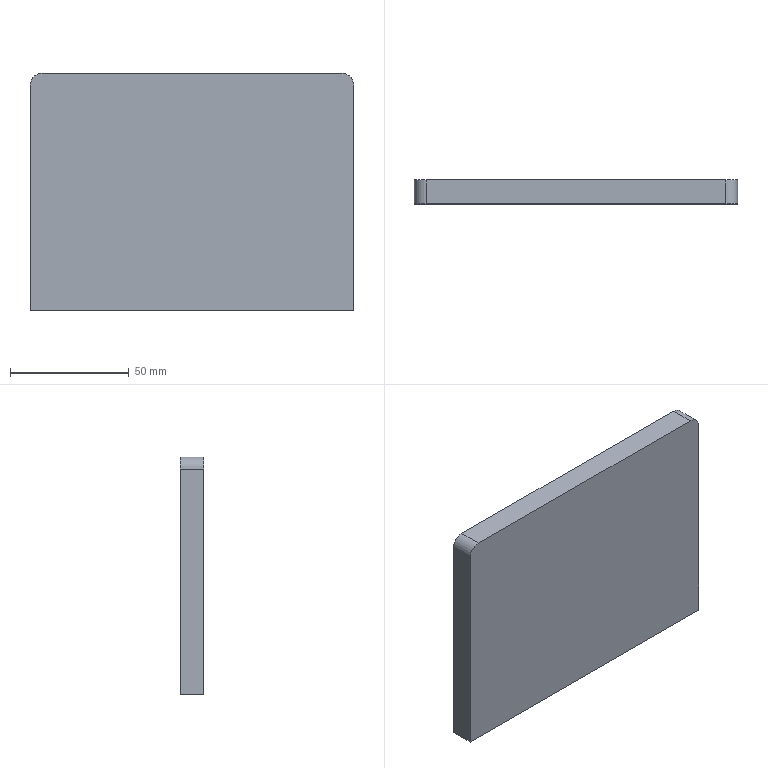Part | STEP file | 1 solid | 8 faces | box 136 x 10 x 100 mm | volume 135893 mm3 | plane 6 | cylinder 2 | commonest cylinder face diameters 10 x2
STEP:
#1=CARTESIAN_POINT('',(0.,0.,0.));
#2=DIRECTION('',(0.,0.,1.));
#3=DIRECTION('',(1.,0.,0.));
#4=AXIS2_PLACEMENT_3D('',#1,#2,#3);
#5=CARTESIAN_POINT('',(-135.863,110.5,353.53));
#6=VERTEX_POINT('',#5);
#7=CARTESIAN_POINT('',(-9.863,110.5,353.53));
#8=VERTEX_POINT('',#7);
#9=CARTESIAN_POINT('',(-72.862,110.5,353.53));
#10=DIRECTION('',(1.,0.,0.));
#11=VECTOR('',#10,1.);
#12=LINE('',#9,#11);
#13=CARTESIAN_POINT('',(-72.862,95.5,353.53));
#14=DIRECTION('',(0.,0.,1.));
#15=DIRECTION('',(1.,0.,0.));
#16=AXIS2_PLACEMENT_3D('',#13,#14,#15);
#17=PLANE('',#16);
#18=CARTESIAN_POINT('',(0.,15.));
#19=DIRECTION('',(1.,0.));
#20=VECTOR('',#19,1.);
#21=LINE('',#18,#20);
#22=(GEOMETRIC_REPRESENTATION_CONTEXT(2)PARAMETRIC_REPRESENTATION_CONTEXT()REPRESENTATION_CONTEXT('',''));
#23=DEFINITIONAL_REPRESENTATION('',(#21),#22);
#24=PCURVE('',#17,#23);
#25=CARTESIAN_POINT('',(-72.862,110.5,253.53));
#26=DIRECTION('',(0.,1.,0.));
#27=DIRECTION('',(0.,0.,1.));
#28=AXIS2_PLACEMENT_3D('',#25,#26,#27);
#29=PLANE('',#28);
#30=CARTESIAN_POINT('',(100.,0.));
#31=DIRECTION('',(0.,1.));
#32=VECTOR('',#31,1.);
#33=LINE('',#30,#32);
#34=(GEOMETRIC_REPRESENTATION_CONTEXT(2)PARAMETRIC_REPRESENTATION_CONTEXT()REPRESENTATION_CONTEXT('',''));
#35=DEFINITIONAL_REPRESENTATION('',(#33),#34);
#36=PCURVE('',#29,#35);
#37=SURFACE_CURVE('',#12,(#24,#36),.PCURVE_S1.);
#38=EDGE_CURVE('',#6,#8,#37,.T.);
#39=ORIENTED_EDGE('',*,*,#38,.F.);
#40=CARTESIAN_POINT('',(-135.863,100.5,353.53));
#41=VERTEX_POINT('',#40);
#42=CARTESIAN_POINT('',(-135.863,95.5,353.53));
#43=DIRECTION('',(0.,-1.,0.));
#44=VECTOR('',#43,1.);
#45=LINE('',#42,#44);
#46=CARTESIAN_POINT('',(-63.,0.));
#47=DIRECTION('',(0.,-1.));
#48=VECTOR('',#47,1.);
#49=LINE('',#46,#48);
#50=(GEOMETRIC_REPRESENTATION_CONTEXT(2)PARAMETRIC_REPRESENTATION_CONTEXT()REPRESENTATION_CONTEXT('',''));
#51=DEFINITIONAL_REPRESENTATION('',(#49),#50);
#52=PCURVE('',#17,#51);
#53=CARTESIAN_POINT('',(-135.863,95.5,348.53));
#54=DIRECTION('',(0.,1.,0.));
#55=DIRECTION('',(0.,0.,1.));
#56=AXIS2_PLACEMENT_3D('',#53,#54,#55);
#57=CYLINDRICAL_SURFACE('',#56,5.);
#58=CARTESIAN_POINT('',(6.283,0.));
#59=DIRECTION('',(0.,-1.));
#60=VECTOR('',#59,1.);
#61=LINE('',#58,#60);
#62=(GEOMETRIC_REPRESENTATION_CONTEXT(2)PARAMETRIC_REPRESENTATION_CONTEXT()REPRESENTATION_CONTEXT('',''));
#63=DEFINITIONAL_REPRESENTATION('',(#61),#62);
#64=PCURVE('',#57,#63);
#65=SURFACE_CURVE('',#45,(#52,#64),.PCURVE_S1.);
#66=EDGE_CURVE('',#6,#41,#65,.T.);
#67=ORIENTED_EDGE('',*,*,#66,.T.);
#68=CARTESIAN_POINT('',(-9.863,100.5,353.53));
#69=VERTEX_POINT('',#68);
#70=CARTESIAN_POINT('',(-72.862,100.5,353.53));
#71=DIRECTION('',(-1.,0.,0.));
#72=VECTOR('',#71,1.);
#73=LINE('',#70,#72);
#74=CARTESIAN_POINT('',(0.,5.));
#75=DIRECTION('',(-1.,0.));
#76=VECTOR('',#75,1.);
#77=LINE('',#74,#76);
#78=(GEOMETRIC_REPRESENTATION_CONTEXT(2)PARAMETRIC_REPRESENTATION_CONTEXT()REPRESENTATION_CONTEXT('',''));
#79=DEFINITIONAL_REPRESENTATION('',(#77),#78);
#80=PCURVE('',#17,#79);
#81=CARTESIAN_POINT('',(-72.862,100.5,253.53));
#82=DIRECTION('',(0.,1.,0.));
#83=DIRECTION('',(0.,0.,1.));
#84=AXIS2_PLACEMENT_3D('',#81,#82,#83);
#85=PLANE('',#84);
#86=CARTESIAN_POINT('',(100.,0.));
#87=DIRECTION('',(0.,-1.));
#88=VECTOR('',#87,1.);
#89=LINE('',#86,#88);
#90=(GEOMETRIC_REPRESENTATION_CONTEXT(2)PARAMETRIC_REPRESENTATION_CONTEXT()REPRESENTATION_CONTEXT('',''));
#91=DEFINITIONAL_REPRESENTATION('',(#89),#90);
#92=PCURVE('',#85,#91);
#93=SURFACE_CURVE('',#73,(#80,#92),.PCURVE_S1.);
#94=EDGE_CURVE('',#69,#41,#93,.T.);
#95=ORIENTED_EDGE('',*,*,#94,.F.);
#96=CARTESIAN_POINT('',(-9.863,95.5,353.53));
#97=DIRECTION('',(0.,1.,0.));
#98=VECTOR('',#97,1.);
#99=LINE('',#96,#98);
#100=CARTESIAN_POINT('',(63.,0.));
#101=DIRECTION('',(0.,1.));
#102=VECTOR('',#101,1.);
#103=LINE('',#100,#102);
#104=(GEOMETRIC_REPRESENTATION_CONTEXT(2)PARAMETRIC_REPRESENTATION_CONTEXT()REPRESENTATION_CONTEXT('',''));
#105=DEFINITIONAL_REPRESENTATION('',(#103),#104);
#106=PCURVE('',#17,#105);
#107=CARTESIAN_POINT('',(-9.863,95.5,348.53));
#108=DIRECTION('',(0.,-1.,0.));
#109=DIRECTION('',(0.,0.,-1.));
#110=AXIS2_PLACEMENT_3D('',#107,#108,#109);
#111=CYLINDRICAL_SURFACE('',#110,5.);
#112=CARTESIAN_POINT('',(3.142,0.));
#113=DIRECTION('',(0.,-1.));
#114=VECTOR('',#113,1.);
#115=LINE('',#112,#114);
#116=(GEOMETRIC_REPRESENTATION_CONTEXT(2)PARAMETRIC_REPRESENTATION_CONTEXT()REPRESENTATION_CONTEXT('',''));
#117=DEFINITIONAL_REPRESENTATION('',(#115),#116);
#118=PCURVE('',#111,#117);
#119=SURFACE_CURVE('',#99,(#106,#118),.PCURVE_S1.);
#120=EDGE_CURVE('',#69,#8,#119,.T.);
#121=ORIENTED_EDGE('',*,*,#120,.T.);
#122=EDGE_LOOP('',(#39,#67,#95,#121));
#123=FACE_BOUND('',#122,.T.);
#124=ADVANCED_FACE('',(#123),#17,.T.);
#125=ORIENTED_EDGE('',*,*,#94,.T.);
#126=CARTESIAN_POINT('',(-140.863,100.5,348.53));
#127=VERTEX_POINT('',#126);
#128=CARTESIAN_POINT('',(-135.863,100.5,348.53));
#129=DIRECTION('',(0.,-1.,0.));
#130=DIRECTION('',(0.,0.,1.));
#131=AXIS2_PLACEMENT_3D('',#128,#129,#130);
#132=CIRCLE('',#131,5.);
#133=CARTESIAN_POINT('',(100.,-63.));
#134=CARTESIAN_POINT('',(100.,-71.66));
#135=CARTESIAN_POINT('',(92.5,-67.33));
#136=CARTESIAN_POINT('',(85.,-63.));
#137=CARTESIAN_POINT('',(92.5,-58.67));
#138=CARTESIAN_POINT('',(100.,-54.34));
#139=CARTESIAN_POINT('',(100.,-63.));
#140=(BOUNDED_CURVE()B_SPLINE_CURVE(2,(#133,#134,#135,#136,#137,#138,#139),.UNSPECIFIED.,.T.,.F.)B_SPLINE_CURVE_WITH_KNOTS((1,2,2,2,2,1),(-2.094,0.,2.094,4.189,6.283,8.378),.UNSPECIFIED.)CURVE()GEOMETRIC_REPRESENTATION_ITEM()RATIONAL_B_SPLINE_CURVE((1.,0.5,1.,0.5,1.,0.5,1.))REPRESENTATION_ITEM(''));
#141=(GEOMETRIC_REPRESENTATION_CONTEXT(2)PARAMETRIC_REPRESENTATION_CONTEXT()REPRESENTATION_CONTEXT('',''));
#142=DEFINITIONAL_REPRESENTATION('',(#140),#141);
#143=PCURVE('',#85,#142);
#144=CARTESIAN_POINT('',(6.283,5.));
#145=DIRECTION('',(-1.,0.));
#146=VECTOR('',#145,1.);
#147=LINE('',#144,#146);
#148=(GEOMETRIC_REPRESENTATION_CONTEXT(2)PARAMETRIC_REPRESENTATION_CONTEXT()REPRESENTATION_CONTEXT('',''));
#149=DEFINITIONAL_REPRESENTATION('',(#147),#148);
#150=PCURVE('',#57,#149);
#151=SURFACE_CURVE('',#132,(#143,#150),.PCURVE_S1.);
#152=EDGE_CURVE('',#41,#127,#151,.T.);
#153=ORIENTED_EDGE('',*,*,#152,.T.);
#154=CARTESIAN_POINT('',(-140.863,100.5,253.53));
#155=VERTEX_POINT('',#154);
#156=CARTESIAN_POINT('',(-140.863,100.5,253.53));
#157=DIRECTION('',(0.,0.,1.));
#158=VECTOR('',#157,1.);
#159=LINE('',#156,#158);
#160=CARTESIAN_POINT('',(0.,-68.));
#161=DIRECTION('',(1.,0.));
#162=VECTOR('',#161,1.);
#163=LINE('',#160,#162);
#164=(GEOMETRIC_REPRESENTATION_CONTEXT(2)PARAMETRIC_REPRESENTATION_CONTEXT()REPRESENTATION_CONTEXT('',''));
#165=DEFINITIONAL_REPRESENTATION('',(#163),#164);
#166=PCURVE('',#85,#165);
#167=CARTESIAN_POINT('',(-140.863,95.5,253.53));
#168=DIRECTION('',(-1.,0.,0.));
#169=DIRECTION('',(0.,0.,1.));
#170=AXIS2_PLACEMENT_3D('',#167,#168,#169);
#171=PLANE('',#170);
#172=CARTESIAN_POINT('',(0.,5.));
#173=DIRECTION('',(1.,0.));
#174=VECTOR('',#173,1.);
#175=LINE('',#172,#174);
#176=(GEOMETRIC_REPRESENTATION_CONTEXT(2)PARAMETRIC_REPRESENTATION_CONTEXT()REPRESENTATION_CONTEXT('',''));
#177=DEFINITIONAL_REPRESENTATION('',(#175),#176);
#178=PCURVE('',#171,#177);
#179=SURFACE_CURVE('',#159,(#166,#178),.PCURVE_S1.);
#180=EDGE_CURVE('',#155,#127,#179,.T.);
#181=ORIENTED_EDGE('',*,*,#180,.F.);
#182=CARTESIAN_POINT('',(-4.862,100.5,253.53));
#183=VERTEX_POINT('',#182);
#184=CARTESIAN_POINT('',(-72.862,100.5,253.53));
#185=DIRECTION('',(1.,0.,0.));
#186=VECTOR('',#185,1.);
#187=LINE('',#184,#186);
#188=CARTESIAN_POINT('',(0.,0.));
#189=DIRECTION('',(0.,1.));
#190=VECTOR('',#189,1.);
#191=LINE('',#188,#190);
#192=(GEOMETRIC_REPRESENTATION_CONTEXT(2)PARAMETRIC_REPRESENTATION_CONTEXT()REPRESENTATION_CONTEXT('',''));
#193=DEFINITIONAL_REPRESENTATION('',(#191),#192);
#194=PCURVE('',#85,#193);
#195=CARTESIAN_POINT('',(-72.862,95.5,253.53));
#196=DIRECTION('',(0.,0.,-1.));
#197=DIRECTION('',(-1.,0.,0.));
#198=AXIS2_PLACEMENT_3D('',#195,#196,#197);
#199=PLANE('',#198);
#200=CARTESIAN_POINT('',(0.,5.));
#201=DIRECTION('',(-1.,0.));
#202=VECTOR('',#201,1.);
#203=LINE('',#200,#202);
#204=(GEOMETRIC_REPRESENTATION_CONTEXT(2)PARAMETRIC_REPRESENTATION_CONTEXT()REPRESENTATION_CONTEXT('',''));
#205=DEFINITIONAL_REPRESENTATION('',(#203),#204);
#206=PCURVE('',#199,#205);
#207=SURFACE_CURVE('',#187,(#194,#206),.PCURVE_S1.);
#208=EDGE_CURVE('',#155,#183,#207,.T.);
#209=ORIENTED_EDGE('',*,*,#208,.T.);
#210=CARTESIAN_POINT('',(-4.862,100.5,348.53));
#211=VERTEX_POINT('',#210);
#212=CARTESIAN_POINT('',(-4.862,100.5,253.53));
#213=DIRECTION('',(0.,0.,1.));
#214=VECTOR('',#213,1.);
#215=LINE('',#212,#214);
#216=CARTESIAN_POINT('',(0.,68.));
#217=DIRECTION('',(1.,0.));
#218=VECTOR('',#217,1.);
#219=LINE('',#216,#218);
#220=(GEOMETRIC_REPRESENTATION_CONTEXT(2)PARAMETRIC_REPRESENTATION_CONTEXT()REPRESENTATION_CONTEXT('',''));
#221=DEFINITIONAL_REPRESENTATION('',(#219),#220);
#222=PCURVE('',#85,#221);
#223=CARTESIAN_POINT('',(-4.862,95.5,253.53));
#224=DIRECTION('',(1.,0.,0.));
#225=DIRECTION('',(0.,0.,-1.));
#226=AXIS2_PLACEMENT_3D('',#223,#224,#225);
#227=PLANE('',#226);
#228=CARTESIAN_POINT('',(0.,5.));
#229=DIRECTION('',(-1.,0.));
#230=VECTOR('',#229,1.);
#231=LINE('',#228,#230);
#232=(GEOMETRIC_REPRESENTATION_CONTEXT(2)PARAMETRIC_REPRESENTATION_CONTEXT()REPRESENTATION_CONTEXT('',''));
#233=DEFINITIONAL_REPRESENTATION('',(#231),#232);
#234=PCURVE('',#227,#233);
#235=SURFACE_CURVE('',#215,(#222,#234),.PCURVE_S1.);
#236=EDGE_CURVE('',#183,#211,#235,.T.);
#237=ORIENTED_EDGE('',*,*,#236,.T.);
#238=CARTESIAN_POINT('',(-9.863,100.5,348.53));
#239=DIRECTION('',(0.,-1.,0.));
#240=DIRECTION('',(0.,0.,1.));
#241=AXIS2_PLACEMENT_3D('',#238,#239,#240);
#242=CIRCLE('',#241,5.);
#243=CARTESIAN_POINT('',(100.,63.));
#244=CARTESIAN_POINT('',(100.,54.34));
#245=CARTESIAN_POINT('',(92.5,58.67));
#246=CARTESIAN_POINT('',(85.,63.));
#247=CARTESIAN_POINT('',(92.5,67.33));
#248=CARTESIAN_POINT('',(100.,71.66));
#249=CARTESIAN_POINT('',(100.,63.));
#250=(BOUNDED_CURVE()B_SPLINE_CURVE(2,(#243,#244,#245,#246,#247,#248,#249),.UNSPECIFIED.,.T.,.F.)B_SPLINE_CURVE_WITH_KNOTS((1,2,2,2,2,1),(-2.094,0.,2.094,4.189,6.283,8.378),.UNSPECIFIED.)CURVE()GEOMETRIC_REPRESENTATION_ITEM()RATIONAL_B_SPLINE_CURVE((1.,0.5,1.,0.5,1.,0.5,1.))REPRESENTATION_ITEM(''));
#251=(GEOMETRIC_REPRESENTATION_CONTEXT(2)PARAMETRIC_REPRESENTATION_CONTEXT()REPRESENTATION_CONTEXT('',''));
#252=DEFINITIONAL_REPRESENTATION('',(#250),#251);
#253=PCURVE('',#85,#252);
#254=CARTESIAN_POINT('',(-3.142,-5.));
#255=DIRECTION('',(1.,0.));
#256=VECTOR('',#255,1.);
#257=LINE('',#254,#256);
#258=(GEOMETRIC_REPRESENTATION_CONTEXT(2)PARAMETRIC_REPRESENTATION_CONTEXT()REPRESENTATION_CONTEXT('',''));
#259=DEFINITIONAL_REPRESENTATION('',(#257),#258);
#260=PCURVE('',#111,#259);
#261=SURFACE_CURVE('',#242,(#253,#260),.PCURVE_S1.);
#262=EDGE_CURVE('',#211,#69,#261,.T.);
#263=ORIENTED_EDGE('',*,*,#262,.T.);
#264=EDGE_LOOP('',(#125,#153,#181,#209,#237,#263));
#265=FACE_BOUND('',#264,.T.);
#266=ADVANCED_FACE('',(#265),#85,.F.);
#267=ORIENTED_EDGE('',*,*,#180,.T.);
#268=CARTESIAN_POINT('',(-140.863,110.5,348.53));
#269=VERTEX_POINT('',#268);
#270=CARTESIAN_POINT('',(-140.863,95.5,348.53));
#271=DIRECTION('',(0.,1.,0.));
#272=VECTOR('',#271,1.);
#273=LINE('',#270,#272);
#274=CARTESIAN_POINT('',(95.,0.));
#275=DIRECTION('',(0.,1.));
#276=VECTOR('',#275,1.);
#277=LINE('',#274,#276);
#278=(GEOMETRIC_REPRESENTATION_CONTEXT(2)PARAMETRIC_REPRESENTATION_CONTEXT()REPRESENTATION_CONTEXT('',''));
#279=DEFINITIONAL_REPRESENTATION('',(#277),#278);
#280=PCURVE('',#171,#279);
#281=CARTESIAN_POINT('',(4.712,0.));
#282=DIRECTION('',(0.,1.));
#283=VECTOR('',#282,1.);
#284=LINE('',#281,#283);
#285=(GEOMETRIC_REPRESENTATION_CONTEXT(2)PARAMETRIC_REPRESENTATION_CONTEXT()REPRESENTATION_CONTEXT('',''));
#286=DEFINITIONAL_REPRESENTATION('',(#284),#285);
#287=PCURVE('',#57,#286);
#288=SURFACE_CURVE('',#273,(#280,#287),.PCURVE_S1.);
#289=EDGE_CURVE('',#127,#269,#288,.T.);
#290=ORIENTED_EDGE('',*,*,#289,.T.);
#291=CARTESIAN_POINT('',(-140.863,110.5,253.53));
#292=VERTEX_POINT('',#291);
#293=CARTESIAN_POINT('',(-140.863,110.5,253.53));
#294=DIRECTION('',(0.,0.,1.));
#295=VECTOR('',#294,1.);
#296=LINE('',#293,#295);
#297=CARTESIAN_POINT('',(0.,15.));
#298=DIRECTION('',(1.,0.));
#299=VECTOR('',#298,1.);
#300=LINE('',#297,#299);
#301=(GEOMETRIC_REPRESENTATION_CONTEXT(2)PARAMETRIC_REPRESENTATION_CONTEXT()REPRESENTATION_CONTEXT('',''));
#302=DEFINITIONAL_REPRESENTATION('',(#300),#301);
#303=PCURVE('',#171,#302);
#304=CARTESIAN_POINT('',(0.,-68.));
#305=DIRECTION('',(1.,0.));
#306=VECTOR('',#305,1.);
#307=LINE('',#304,#306);
#308=(GEOMETRIC_REPRESENTATION_CONTEXT(2)PARAMETRIC_REPRESENTATION_CONTEXT()REPRESENTATION_CONTEXT('',''));
#309=DEFINITIONAL_REPRESENTATION('',(#307),#308);
#310=PCURVE('',#29,#309);
#311=SURFACE_CURVE('',#296,(#303,#310),.PCURVE_S1.);
#312=EDGE_CURVE('',#292,#269,#311,.T.);
#313=ORIENTED_EDGE('',*,*,#312,.F.);
#314=CARTESIAN_POINT('',(-140.863,95.5,253.53));
#315=DIRECTION('',(0.,-1.,0.));
#316=VECTOR('',#315,1.);
#317=LINE('',#314,#316);
#318=CARTESIAN_POINT('',(0.,0.));
#319=DIRECTION('',(0.,-1.));
#320=VECTOR('',#319,1.);
#321=LINE('',#318,#320);
#322=(GEOMETRIC_REPRESENTATION_CONTEXT(2)PARAMETRIC_REPRESENTATION_CONTEXT()REPRESENTATION_CONTEXT('',''));
#323=DEFINITIONAL_REPRESENTATION('',(#321),#322);
#324=PCURVE('',#171,#323);
#325=CARTESIAN_POINT('',(68.,0.));
#326=DIRECTION('',(0.,-1.));
#327=VECTOR('',#326,1.);
#328=LINE('',#325,#327);
#329=(GEOMETRIC_REPRESENTATION_CONTEXT(2)PARAMETRIC_REPRESENTATION_CONTEXT()REPRESENTATION_CONTEXT('',''));
#330=DEFINITIONAL_REPRESENTATION('',(#328),#329);
#331=PCURVE('',#199,#330);
#332=SURFACE_CURVE('',#317,(#324,#331),.PCURVE_S1.);
#333=EDGE_CURVE('',#292,#155,#332,.T.);
#334=ORIENTED_EDGE('',*,*,#333,.T.);
#335=EDGE_LOOP('',(#267,#290,#313,#334));
#336=FACE_BOUND('',#335,.T.);
#337=ADVANCED_FACE('',(#336),#171,.T.);
#338=ORIENTED_EDGE('',*,*,#312,.T.);
#339=CARTESIAN_POINT('',(-135.863,110.5,348.53));
#340=DIRECTION('',(0.,1.,0.));
#341=DIRECTION('',(0.,0.,1.));
#342=AXIS2_PLACEMENT_3D('',#339,#340,#341);
#343=CIRCLE('',#342,5.);
#344=CARTESIAN_POINT('',(95.,-63.));
#345=DIRECTION('',(1.,0.));
#346=AXIS2_PLACEMENT_2D('',#344,#345);
#347=CIRCLE('',#346,5.);
#348=(GEOMETRIC_REPRESENTATION_CONTEXT(2)PARAMETRIC_REPRESENTATION_CONTEXT()REPRESENTATION_CONTEXT('',''));
#349=DEFINITIONAL_REPRESENTATION('',(#347),#348);
#350=PCURVE('',#29,#349);
#351=CARTESIAN_POINT('',(0.,15.));
#352=DIRECTION('',(1.,0.));
#353=VECTOR('',#352,1.);
#354=LINE('',#351,#353);
#355=(GEOMETRIC_REPRESENTATION_CONTEXT(2)PARAMETRIC_REPRESENTATION_CONTEXT()REPRESENTATION_CONTEXT('',''));
#356=DEFINITIONAL_REPRESENTATION('',(#354),#355);
#357=PCURVE('',#57,#356);
#358=SURFACE_CURVE('',#343,(#350,#357),.PCURVE_S1.);
#359=EDGE_CURVE('',#269,#6,#358,.T.);
#360=ORIENTED_EDGE('',*,*,#359,.T.);
#361=ORIENTED_EDGE('',*,*,#38,.T.);
#362=CARTESIAN_POINT('',(-4.862,110.5,348.53));
#363=VERTEX_POINT('',#362);
#364=CARTESIAN_POINT('',(-9.863,110.5,348.53));
#365=DIRECTION('',(0.,1.,0.));
#366=DIRECTION('',(0.,0.,1.));
#367=AXIS2_PLACEMENT_3D('',#364,#365,#366);
#368=CIRCLE('',#367,5.);
#369=CARTESIAN_POINT('',(95.,63.));
#370=DIRECTION('',(1.,0.));
#371=AXIS2_PLACEMENT_2D('',#369,#370);
#372=CIRCLE('',#371,5.);
#373=(GEOMETRIC_REPRESENTATION_CONTEXT(2)PARAMETRIC_REPRESENTATION_CONTEXT()REPRESENTATION_CONTEXT('',''));
#374=DEFINITIONAL_REPRESENTATION('',(#372),#373);
#375=PCURVE('',#29,#374);
#376=CARTESIAN_POINT('',(3.142,-15.));
#377=DIRECTION('',(-1.,0.));
#378=VECTOR('',#377,1.);
#379=LINE('',#376,#378);
#380=(GEOMETRIC_REPRESENTATION_CONTEXT(2)PARAMETRIC_REPRESENTATION_CONTEXT()REPRESENTATION_CONTEXT('',''));
#381=DEFINITIONAL_REPRESENTATION('',(#379),#380);
#382=PCURVE('',#111,#381);
#383=SURFACE_CURVE('',#368,(#375,#382),.PCURVE_S1.);
#384=EDGE_CURVE('',#8,#363,#383,.T.);
#385=ORIENTED_EDGE('',*,*,#384,.T.);
#386=CARTESIAN_POINT('',(-4.862,110.5,253.53));
#387=VERTEX_POINT('',#386);
#388=CARTESIAN_POINT('',(-4.862,110.5,253.53));
#389=DIRECTION('',(0.,0.,1.));
#390=VECTOR('',#389,1.);
#391=LINE('',#388,#390);
#392=CARTESIAN_POINT('',(0.,68.));
#393=DIRECTION('',(1.,0.));
#394=VECTOR('',#393,1.);
#395=LINE('',#392,#394);
#396=(GEOMETRIC_REPRESENTATION_CONTEXT(2)PARAMETRIC_REPRESENTATION_CONTEXT()REPRESENTATION_CONTEXT('',''));
#397=DEFINITIONAL_REPRESENTATION('',(#395),#396);
#398=PCURVE('',#29,#397);
#399=CARTESIAN_POINT('',(0.,15.));
#400=DIRECTION('',(-1.,0.));
#401=VECTOR('',#400,1.);
#402=LINE('',#399,#401);
#403=(GEOMETRIC_REPRESENTATION_CONTEXT(2)PARAMETRIC_REPRESENTATION_CONTEXT()REPRESENTATION_CONTEXT('',''));
#404=DEFINITIONAL_REPRESENTATION('',(#402),#403);
#405=PCURVE('',#227,#404);
#406=SURFACE_CURVE('',#391,(#398,#405),.PCURVE_S1.);
#407=EDGE_CURVE('',#387,#363,#406,.T.);
#408=ORIENTED_EDGE('',*,*,#407,.F.);
#409=CARTESIAN_POINT('',(-72.862,110.5,253.53));
#410=DIRECTION('',(-1.,0.,0.));
#411=VECTOR('',#410,1.);
#412=LINE('',#409,#411);
#413=CARTESIAN_POINT('',(0.,0.));
#414=DIRECTION('',(0.,-1.));
#415=VECTOR('',#414,1.);
#416=LINE('',#413,#415);
#417=(GEOMETRIC_REPRESENTATION_CONTEXT(2)PARAMETRIC_REPRESENTATION_CONTEXT()REPRESENTATION_CONTEXT('',''));
#418=DEFINITIONAL_REPRESENTATION('',(#416),#417);
#419=PCURVE('',#29,#418);
#420=CARTESIAN_POINT('',(0.,15.));
#421=DIRECTION('',(1.,0.));
#422=VECTOR('',#421,1.);
#423=LINE('',#420,#422);
#424=(GEOMETRIC_REPRESENTATION_CONTEXT(2)PARAMETRIC_REPRESENTATION_CONTEXT()REPRESENTATION_CONTEXT('',''));
#425=DEFINITIONAL_REPRESENTATION('',(#423),#424);
#426=PCURVE('',#199,#425);
#427=SURFACE_CURVE('',#412,(#419,#426),.PCURVE_S1.);
#428=EDGE_CURVE('',#387,#292,#427,.T.);
#429=ORIENTED_EDGE('',*,*,#428,.T.);
#430=EDGE_LOOP('',(#338,#360,#361,#385,#408,#429));
#431=FACE_BOUND('',#430,.T.);
#432=ADVANCED_FACE('',(#431),#29,.T.);
#433=CARTESIAN_POINT('',(-4.862,95.5,253.53));
#434=DIRECTION('',(0.,1.,0.));
#435=VECTOR('',#434,1.);
#436=LINE('',#433,#435);
#437=CARTESIAN_POINT('',(-68.,0.));
#438=DIRECTION('',(0.,1.));
#439=VECTOR('',#438,1.);
#440=LINE('',#437,#439);
#441=(GEOMETRIC_REPRESENTATION_CONTEXT(2)PARAMETRIC_REPRESENTATION_CONTEXT()REPRESENTATION_CONTEXT('',''));
#442=DEFINITIONAL_REPRESENTATION('',(#440),#441);
#443=PCURVE('',#199,#442);
#444=CARTESIAN_POINT('',(0.,0.));
#445=DIRECTION('',(0.,1.));
#446=VECTOR('',#445,1.);
#447=LINE('',#444,#446);
#448=(GEOMETRIC_REPRESENTATION_CONTEXT(2)PARAMETRIC_REPRESENTATION_CONTEXT()REPRESENTATION_CONTEXT('',''));
#449=DEFINITIONAL_REPRESENTATION('',(#447),#448);
#450=PCURVE('',#227,#449);
#451=SURFACE_CURVE('',#436,(#443,#450),.PCURVE_S1.);
#452=EDGE_CURVE('',#183,#387,#451,.T.);
#453=ORIENTED_EDGE('',*,*,#452,.F.);
#454=ORIENTED_EDGE('',*,*,#208,.F.);
#455=ORIENTED_EDGE('',*,*,#333,.F.);
#456=ORIENTED_EDGE('',*,*,#428,.F.);
#457=EDGE_LOOP('',(#453,#454,#455,#456));
#458=FACE_BOUND('',#457,.T.);
#459=ADVANCED_FACE('',(#458),#199,.T.);
#460=ORIENTED_EDGE('',*,*,#407,.T.);
#461=CARTESIAN_POINT('',(-4.862,95.5,348.53));
#462=DIRECTION('',(0.,-1.,0.));
#463=VECTOR('',#462,1.);
#464=LINE('',#461,#463);
#465=CARTESIAN_POINT('',(-95.,0.));
#466=DIRECTION('',(0.,-1.));
#467=VECTOR('',#466,1.);
#468=LINE('',#465,#467);
#469=(GEOMETRIC_REPRESENTATION_CONTEXT(2)PARAMETRIC_REPRESENTATION_CONTEXT()REPRESENTATION_CONTEXT('',''));
#470=DEFINITIONAL_REPRESENTATION('',(#468),#469);
#471=PCURVE('',#227,#470);
#472=CARTESIAN_POINT('',(1.571,0.));
#473=DIRECTION('',(0.,1.));
#474=VECTOR('',#473,1.);
#475=LINE('',#472,#474);
#476=(GEOMETRIC_REPRESENTATION_CONTEXT(2)PARAMETRIC_REPRESENTATION_CONTEXT()REPRESENTATION_CONTEXT('',''));
#477=DEFINITIONAL_REPRESENTATION('',(#475),#476);
#478=PCURVE('',#111,#477);
#479=SURFACE_CURVE('',#464,(#471,#478),.PCURVE_S1.);
#480=EDGE_CURVE('',#363,#211,#479,.T.);
#481=ORIENTED_EDGE('',*,*,#480,.T.);
#482=ORIENTED_EDGE('',*,*,#236,.F.);
#483=ORIENTED_EDGE('',*,*,#452,.T.);
#484=EDGE_LOOP('',(#460,#481,#482,#483));
#485=FACE_BOUND('',#484,.T.);
#486=ADVANCED_FACE('',(#485),#227,.T.);
#487=ORIENTED_EDGE('',*,*,#152,.F.);
#488=ORIENTED_EDGE('',*,*,#66,.F.);
#489=ORIENTED_EDGE('',*,*,#359,.F.);
#490=ORIENTED_EDGE('',*,*,#289,.F.);
#491=EDGE_LOOP('',(#487,#488,#489,#490));
#492=FACE_BOUND('',#491,.T.);
#493=ADVANCED_FACE('',(#492),#57,.T.);
#494=ORIENTED_EDGE('',*,*,#384,.F.);
#495=ORIENTED_EDGE('',*,*,#120,.F.);
#496=ORIENTED_EDGE('',*,*,#262,.F.);
#497=ORIENTED_EDGE('',*,*,#480,.F.);
#498=EDGE_LOOP('',(#494,#495,#496,#497));
#499=FACE_BOUND('',#498,.T.);
#500=ADVANCED_FACE('',(#499),#111,.T.);
#501=CLOSED_SHELL('',(#124,#266,#337,#432,#459,#486,#493,#500));
#502=MANIFOLD_SOLID_BREP('',#501);
#503=(LENGTH_UNIT()NAMED_UNIT(*)SI_UNIT(.MILLI.,.METRE.));
#504=UNCERTAINTY_MEASURE_WITH_UNIT(LENGTH_MEASURE(0.0000001),#503,'','');
#505=(NAMED_UNIT(*)PLANE_ANGLE_UNIT()SI_UNIT($,.RADIAN.));
#506=(NAMED_UNIT(*)SI_UNIT($,.STERADIAN.)SOLID_ANGLE_UNIT());
#507=(GEOMETRIC_REPRESENTATION_CONTEXT(3)GLOBAL_UNCERTAINTY_ASSIGNED_CONTEXT((#504))GLOBAL_UNIT_ASSIGNED_CONTEXT((#503,#505,#506))REPRESENTATION_CONTEXT('',''));
#508=ADVANCED_BREP_SHAPE_REPRESENTATION('',(#4,#502),#507);